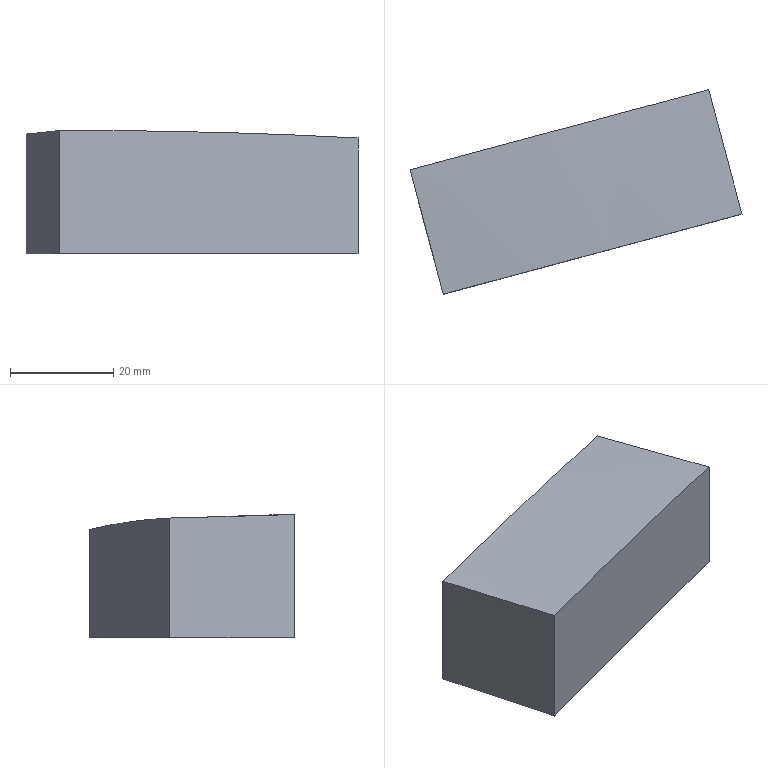Part | NX | features solid 2 | 1 solid | 6 faces | box 64.426 x 39.677 x 23.874 mm | volume 34310 mm3 | plane 5 | spline 1
STEP:
#1=CARTESIAN_POINT('',(-935.741,-113.852,45.));
#2=VERTEX_POINT('',#1);
#3=CARTESIAN_POINT('',(-929.27,-138.001,45.));
#4=VERTEX_POINT('',#3);
#5=CARTESIAN_POINT('',(-935.741,-113.852,45.));
#6=DIRECTION('',(0.2588,-0.9659,0.));
#7=VECTOR('',#6,1000.);
#8=LINE('',#5,#7);
#9=EDGE_CURVE('',#2,#4,#8,.T.);
#10=ORIENTED_EDGE('',*,*,#9,.F.);
#11=CARTESIAN_POINT('',(-935.741,-113.852,65.969));
#12=VERTEX_POINT('',#11);
#13=CARTESIAN_POINT('',(-935.741,-113.852,-10.));
#14=DIRECTION('',(0.,0.,1.));
#15=VECTOR('',#14,1000.);
#16=LINE('',#13,#15);
#17=EDGE_CURVE('',#2,#12,#16,.T.);
#18=ORIENTED_EDGE('',*,*,#17,.T.);
#19=CARTESIAN_POINT('',(-929.27,-138.001,67.427));
#20=VERTEX_POINT('',#19);
#21=CARTESIAN_POINT('',(-935.741,-113.852,65.969));
#22=CARTESIAN_POINT('',(-933.584,-121.902,66.456));
#23=CARTESIAN_POINT('',(-931.427,-129.951,66.94));
#24=CARTESIAN_POINT('',(-929.27,-138.001,67.427));
#25=B_SPLINE_CURVE_WITH_KNOTS('',3,(#21,#22,#23,#24),.UNSPECIFIED.,.F.,.F.,(4,4),(0.,0.02504),.UNSPECIFIED.);
#26=EDGE_CURVE('',#12,#20,#25,.T.);
#27=ORIENTED_EDGE('',*,*,#26,.T.);
#28=CARTESIAN_POINT('',(-929.27,-138.001,-10.));
#29=DIRECTION('',(0.,0.,1.));
#30=VECTOR('',#29,1000.);
#31=LINE('',#28,#30);
#32=EDGE_CURVE('',#4,#20,#31,.T.);
#33=ORIENTED_EDGE('',*,*,#32,.F.);
#34=EDGE_LOOP('',(#10,#18,#27,#33));
#35=FACE_BOUND('',#34,.T.);
#36=CARTESIAN_POINT('',(-935.741,-113.852,-10.));
#37=DIRECTION('',(-0.9659,-0.2588,0.));
#38=DIRECTION('',(0.2588,-0.9659,0.));
#39=AXIS2_PLACEMENT_3D('',#36,#37,#38);
#40=PLANE('',#39);
#41=ADVANCED_FACE('',(#35),#40,.F.);
#42=CARTESIAN_POINT('',(-993.696,-129.382,45.));
#43=VERTEX_POINT('',#42);
#44=CARTESIAN_POINT('',(-993.696,-129.382,68.182));
#45=VERTEX_POINT('',#44);
#46=CARTESIAN_POINT('',(-993.696,-129.382,-10.));
#47=DIRECTION('',(0.,0.,1.));
#48=VECTOR('',#47,1000.);
#49=LINE('',#46,#48);
#50=EDGE_CURVE('',#43,#45,#49,.T.);
#51=ORIENTED_EDGE('',*,*,#50,.F.);
#52=CARTESIAN_POINT('',(-987.226,-153.53,45.));
#53=VERTEX_POINT('',#52);
#54=CARTESIAN_POINT('',(-993.696,-129.382,45.));
#55=DIRECTION('',(0.2588,-0.9659,0.));
#56=VECTOR('',#55,1000.);
#57=LINE('',#54,#56);
#58=EDGE_CURVE('',#43,#53,#57,.T.);
#59=ORIENTED_EDGE('',*,*,#58,.T.);
#60=CARTESIAN_POINT('',(-987.226,-153.53,68.873));
#61=VERTEX_POINT('',#60);
#62=CARTESIAN_POINT('',(-987.226,-153.53,-10.));
#63=DIRECTION('',(0.,0.,1.));
#64=VECTOR('',#63,1000.);
#65=LINE('',#62,#64);
#66=EDGE_CURVE('',#53,#61,#65,.T.);
#67=ORIENTED_EDGE('',*,*,#66,.T.);
#68=CARTESIAN_POINT('',(-993.696,-129.382,68.182));
#69=CARTESIAN_POINT('',(-991.54,-137.43,68.431));
#70=CARTESIAN_POINT('',(-989.382,-145.482,68.569));
#71=CARTESIAN_POINT('',(-987.226,-153.53,68.873));
#72=B_SPLINE_CURVE_WITH_KNOTS('',3,(#68,#69,#70,#71),.UNSPECIFIED.,.F.,.F.,(4,4),(0.,0.02501),.UNSPECIFIED.);
#73=EDGE_CURVE('',#45,#61,#72,.T.);
#74=ORIENTED_EDGE('',*,*,#73,.F.);
#75=EDGE_LOOP('',(#51,#59,#67,#74));
#76=FACE_BOUND('',#75,.T.);
#77=CARTESIAN_POINT('',(-993.696,-129.382,-10.));
#78=DIRECTION('',(-0.9659,-0.2588,0.));
#79=DIRECTION('',(0.2588,-0.9659,0.));
#80=AXIS2_PLACEMENT_3D('',#77,#78,#79);
#81=PLANE('',#80);
#82=ADVANCED_FACE('',(#76),#81,.T.);
#83=CARTESIAN_POINT('',(-993.696,-129.382,45.));
#84=DIRECTION('',(0.9659,0.2588,0.));
#85=VECTOR('',#84,1000.);
#86=LINE('',#83,#85);
#87=EDGE_CURVE('',#43,#2,#86,.T.);
#88=ORIENTED_EDGE('',*,*,#87,.F.);
#89=ORIENTED_EDGE('',*,*,#50,.T.);
#90=CARTESIAN_POINT('',(-993.696,-129.382,68.182));
#91=CARTESIAN_POINT('',(-984.028,-126.791,68.057));
#92=CARTESIAN_POINT('',(-964.699,-121.612,67.62));
#93=CARTESIAN_POINT('',(-945.391,-116.438,66.584));
#94=CARTESIAN_POINT('',(-935.741,-113.852,65.969));
#95=B_SPLINE_CURVE_WITH_KNOTS('',3,(#90,#91,#92,#93,#94),.UNSPECIFIED.,.F.,.F.,(4,1,4),(0.,0.03002,0.06004),.UNSPECIFIED.);
#96=EDGE_CURVE('',#45,#12,#95,.T.);
#97=ORIENTED_EDGE('',*,*,#96,.T.);
#98=ORIENTED_EDGE('',*,*,#17,.F.);
#99=EDGE_LOOP('',(#88,#89,#97,#98));
#100=FACE_BOUND('',#99,.T.);
#101=CARTESIAN_POINT('',(-993.696,-129.382,-10.));
#102=DIRECTION('',(0.2588,-0.9659,0.));
#103=DIRECTION('',(0.,0.,1.));
#104=AXIS2_PLACEMENT_3D('',#101,#102,#103);
#105=PLANE('',#104);
#106=ADVANCED_FACE('',(#100),#105,.F.);
#107=CARTESIAN_POINT('',(-987.226,-153.53,45.));
#108=DIRECTION('',(0.9659,0.2588,0.));
#109=VECTOR('',#108,1000.);
#110=LINE('',#107,#109);
#111=EDGE_CURVE('',#4,#53,#110,.F.);
#112=ORIENTED_EDGE('',*,*,#111,.F.);
#113=ORIENTED_EDGE('',*,*,#32,.T.);
#114=CARTESIAN_POINT('',(-929.27,-138.001,67.427));
#115=CARTESIAN_POINT('',(-938.924,-140.587,67.925));
#116=CARTESIAN_POINT('',(-958.234,-145.761,68.731));
#117=CARTESIAN_POINT('',(-977.561,-150.94,68.876));
#118=CARTESIAN_POINT('',(-987.226,-153.53,68.873));
#119=B_SPLINE_CURVE_WITH_KNOTS('',3,(#114,#115,#116,#117,#118),.UNSPECIFIED.,.F.,.F.,(4,1,4),(0.,0.03001,0.06002),.UNSPECIFIED.);
#120=EDGE_CURVE('',#20,#61,#119,.T.);
#121=ORIENTED_EDGE('',*,*,#120,.T.);
#122=ORIENTED_EDGE('',*,*,#66,.F.);
#123=EDGE_LOOP('',(#112,#113,#121,#122));
#124=FACE_BOUND('',#123,.T.);
#125=CARTESIAN_POINT('',(-987.226,-153.53,-10.));
#126=DIRECTION('',(0.2588,-0.9659,0.));
#127=DIRECTION('',(0.,0.,1.));
#128=AXIS2_PLACEMENT_3D('',#125,#126,#127);
#129=PLANE('',#128);
#130=ADVANCED_FACE('',(#124),#129,.T.);
#131=ORIENTED_EDGE('',*,*,#26,.F.);
#132=ORIENTED_EDGE('',*,*,#96,.F.);
#133=ORIENTED_EDGE('',*,*,#73,.T.);
#134=ORIENTED_EDGE('',*,*,#120,.F.);
#135=EDGE_LOOP('',(#131,#132,#133,#134));
#136=FACE_BOUND('',#135,.T.);
#137=CARTESIAN_POINT('',(-990.745,-88.742,66.599));
#138=CARTESIAN_POINT('',(-991.244,-92.487,66.806));
#139=CARTESIAN_POINT('',(-992.291,-101.121,67.26));
#140=CARTESIAN_POINT('',(-993.369,-112.833,67.68));
#141=CARTESIAN_POINT('',(-994.011,-123.856,67.993));
#142=CARTESIAN_POINT('',(-994.153,-133.042,68.318));
#143=CARTESIAN_POINT('',(-993.916,-142.159,68.485));
#144=CARTESIAN_POINT('',(-993.635,-148.206,68.637));
#145=CARTESIAN_POINT('',(-993.495,-151.104,68.725));
#146=CARTESIAN_POINT('',(-969.375,-98.352,66.344));
#147=CARTESIAN_POINT('',(-969.873,-102.095,66.585));
#148=CARTESIAN_POINT('',(-970.917,-110.725,67.119));
#149=CARTESIAN_POINT('',(-971.991,-122.429,67.679));
#150=CARTESIAN_POINT('',(-972.63,-133.443,68.143));
#151=CARTESIAN_POINT('',(-972.77,-142.622,68.58));
#152=CARTESIAN_POINT('',(-972.531,-151.731,68.88));
#153=CARTESIAN_POINT('',(-972.249,-157.772,69.132));
#154=CARTESIAN_POINT('',(-972.109,-160.666,69.276));
#155=CARTESIAN_POINT('',(-948.005,-107.962,66.089));
#156=CARTESIAN_POINT('',(-948.502,-111.703,66.363));
#157=CARTESIAN_POINT('',(-949.543,-120.328,66.974));
#158=CARTESIAN_POINT('',(-950.613,-132.025,67.679));
#159=CARTESIAN_POINT('',(-951.248,-143.03,68.3));
#160=CARTESIAN_POINT('',(-951.387,-152.203,68.839));
#161=CARTESIAN_POINT('',(-951.146,-161.303,69.28));
#162=CARTESIAN_POINT('',(-950.863,-167.337,69.632));
#163=CARTESIAN_POINT('',(-950.723,-170.227,69.829));
#164=CARTESIAN_POINT('',(-926.635,-117.571,65.833));
#165=CARTESIAN_POINT('',(-927.131,-121.311,66.141));
#166=CARTESIAN_POINT('',(-928.169,-129.932,66.832));
#167=CARTESIAN_POINT('',(-929.235,-141.621,67.679));
#168=CARTESIAN_POINT('',(-929.867,-152.617,68.449));
#169=CARTESIAN_POINT('',(-930.004,-161.784,69.097));
#170=CARTESIAN_POINT('',(-929.761,-170.874,69.689));
#171=CARTESIAN_POINT('',(-929.477,-176.902,70.141));
#172=CARTESIAN_POINT('',(-929.337,-179.789,70.387));
#173=B_SPLINE_SURFACE_WITH_KNOTS('',3,3,((#137,#138,#139,#140,#141,#142,#143,#144,#145),(#146,#147,#148,#149,#150,#151,#152,#153,#154),(#155,#156,#157,#158,#159,#160,#161,#162,#163),(#164,#165,#166,#167,#168,#169,#170,#171,#172)),.UNSPECIFIED.,.F.,.F.,.F.,(4,4),(4,1,1,1,1,1,4),(0.408,0.7944),(0.692,0.7255,0.7689,0.795,0.821,0.847,0.871),.UNSPECIFIED.);
#174=ADVANCED_FACE('',(#136),#173,.F.);
#175=ORIENTED_EDGE('',*,*,#58,.F.);
#176=ORIENTED_EDGE('',*,*,#87,.T.);
#177=ORIENTED_EDGE('',*,*,#9,.T.);
#178=ORIENTED_EDGE('',*,*,#111,.T.);
#179=EDGE_LOOP('',(#175,#176,#177,#178));
#180=FACE_BOUND('',#179,.T.);
#181=CARTESIAN_POINT('',(-993.696,-129.382,45.));
#182=DIRECTION('',(0.,0.,-1.));
#183=DIRECTION('',(-1.,0.,0.));
#184=AXIS2_PLACEMENT_3D('',#181,#182,#183);
#185=PLANE('',#184);
#186=ADVANCED_FACE('',(#180),#185,.T.);
#187=CLOSED_SHELL('',(#41,#82,#106,#130,#174,#186));
#188=MANIFOLD_SOLID_BREP('',#187);
#189=(LENGTH_UNIT()NAMED_UNIT(*)SI_UNIT(.MILLI.,.METRE.));
#190=UNCERTAINTY_MEASURE_WITH_UNIT(LENGTH_MEASURE(0.0508),#189,'','');
#191=(NAMED_UNIT(*)PLANE_ANGLE_UNIT()SI_UNIT($,.RADIAN.));
#192=(NAMED_UNIT(*)SI_UNIT($,.STERADIAN.)SOLID_ANGLE_UNIT());
#193=(GEOMETRIC_REPRESENTATION_CONTEXT(3)GLOBAL_UNCERTAINTY_ASSIGNED_CONTEXT((#190))GLOBAL_UNIT_ASSIGNED_CONTEXT((#189,#191,#192))REPRESENTATION_CONTEXT('',''));
#194=ADVANCED_BREP_SHAPE_REPRESENTATION('',(#188),#193);